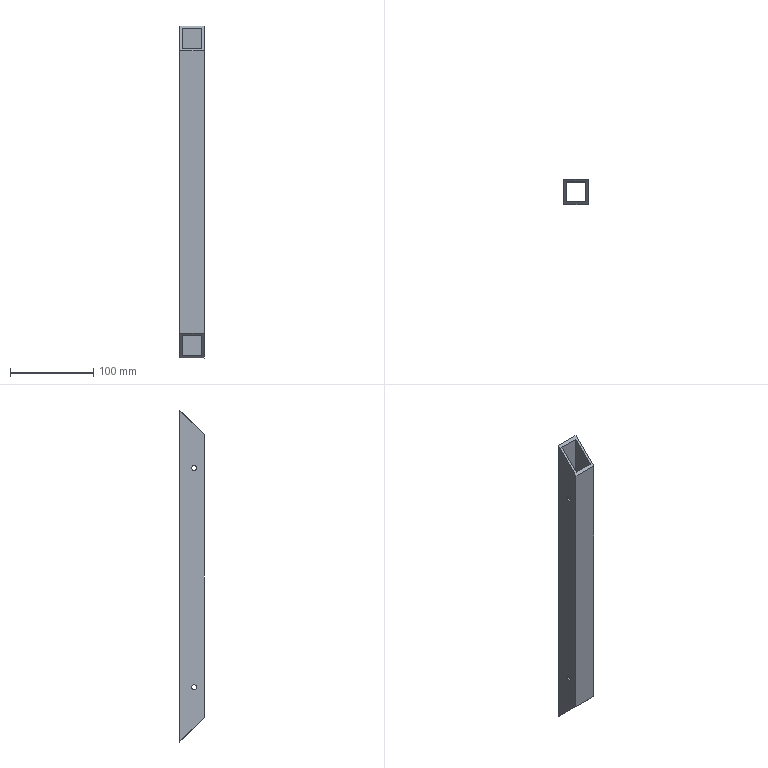Part | SolidWorks | features ICE 4, Extrusion 1 | 1 solid | 18 faces | box 30 x 30 x 400 mm | volume 119541 mm3 | plane 10 | cylinder 8 | commonest cylinder face diameters 6 x8
STEP:
#1=CARTESIAN_POINT('',(-45.142,8.401,333.));
#2=VERTEX_POINT('',#1);
#3=CARTESIAN_POINT('',(-45.142,8.401,327.));
#4=VERTEX_POINT('',#3);
#5=CARTESIAN_POINT('',(-45.142,8.401,330.));
#6=DIRECTION('',(1.,0.,0.));
#7=DIRECTION('',(0.,0.,-1.));
#8=AXIS2_PLACEMENT_3D('',#5,#6,#7);
#9=CIRCLE('',#8,3.);
#10=EDGE_CURVE('',#2,#4,#9,.T.);
#11=ORIENTED_EDGE('',*,*,#10,.F.);
#12=CARTESIAN_POINT('',(-42.142,8.401,333.));
#13=VERTEX_POINT('',#12);
#14=CARTESIAN_POINT('',(-45.142,8.401,333.));
#15=DIRECTION('',(1.,0.,0.));
#16=VECTOR('',#15,1000.);
#17=LINE('',#14,#16);
#18=EDGE_CURVE('',#2,#13,#17,.T.);
#19=ORIENTED_EDGE('',*,*,#18,.T.);
#20=CARTESIAN_POINT('',(-42.142,8.401,327.));
#21=VERTEX_POINT('',#20);
#22=CARTESIAN_POINT('',(-42.142,8.401,330.));
#23=DIRECTION('',(-1.,0.,0.));
#24=DIRECTION('',(0.,0.,1.));
#25=AXIS2_PLACEMENT_3D('',#22,#23,#24);
#26=CIRCLE('',#25,3.);
#27=EDGE_CURVE('',#21,#13,#26,.T.);
#28=ORIENTED_EDGE('',*,*,#27,.F.);
#29=CARTESIAN_POINT('',(-45.142,8.401,327.));
#30=DIRECTION('',(1.,0.,0.));
#31=VECTOR('',#30,1000.);
#32=LINE('',#29,#31);
#33=EDGE_CURVE('',#4,#21,#32,.T.);
#34=ORIENTED_EDGE('',*,*,#33,.F.);
#35=EDGE_LOOP('',(#11,#19,#28,#34));
#36=FACE_OUTER_BOUND('',#35,.T.);
#37=CARTESIAN_POINT('',(-45.142,8.401,330.));
#38=DIRECTION('',(1.,0.,0.));
#39=DIRECTION('',(0.,0.,-1.));
#40=AXIS2_PLACEMENT_3D('',#37,#38,#39);
#41=CYLINDRICAL_SURFACE('',#40,3.);
#42=ADVANCED_FACE('',(#36),#41,.F.);
#43=CARTESIAN_POINT('',(-45.142,8.401,69.));
#44=VERTEX_POINT('',#43);
#45=CARTESIAN_POINT('',(-45.142,8.401,63.));
#46=VERTEX_POINT('',#45);
#47=CARTESIAN_POINT('',(-45.142,8.401,66.));
#48=DIRECTION('',(1.,0.,0.));
#49=DIRECTION('',(0.,0.,-1.));
#50=AXIS2_PLACEMENT_3D('',#47,#48,#49);
#51=CIRCLE('',#50,3.);
#52=EDGE_CURVE('',#44,#46,#51,.T.);
#53=ORIENTED_EDGE('',*,*,#52,.F.);
#54=CARTESIAN_POINT('',(-42.142,8.401,69.));
#55=VERTEX_POINT('',#54);
#56=CARTESIAN_POINT('',(-45.142,8.401,69.));
#57=DIRECTION('',(1.,0.,0.));
#58=VECTOR('',#57,1000.);
#59=LINE('',#56,#58);
#60=EDGE_CURVE('',#44,#55,#59,.T.);
#61=ORIENTED_EDGE('',*,*,#60,.T.);
#62=CARTESIAN_POINT('',(-42.142,8.401,63.));
#63=VERTEX_POINT('',#62);
#64=CARTESIAN_POINT('',(-42.142,8.401,66.));
#65=DIRECTION('',(-1.,0.,0.));
#66=DIRECTION('',(0.,0.,1.));
#67=AXIS2_PLACEMENT_3D('',#64,#65,#66);
#68=CIRCLE('',#67,3.);
#69=EDGE_CURVE('',#63,#55,#68,.T.);
#70=ORIENTED_EDGE('',*,*,#69,.F.);
#71=CARTESIAN_POINT('',(-45.142,8.401,63.));
#72=DIRECTION('',(1.,0.,0.));
#73=VECTOR('',#72,1000.);
#74=LINE('',#71,#73);
#75=EDGE_CURVE('',#46,#63,#74,.T.);
#76=ORIENTED_EDGE('',*,*,#75,.F.);
#77=EDGE_LOOP('',(#53,#61,#70,#76));
#78=FACE_OUTER_BOUND('',#77,.T.);
#79=CARTESIAN_POINT('',(-45.142,8.401,66.));
#80=DIRECTION('',(1.,0.,0.));
#81=DIRECTION('',(0.,0.,-1.));
#82=AXIS2_PLACEMENT_3D('',#79,#80,#81);
#83=CYLINDRICAL_SURFACE('',#82,3.);
#84=ADVANCED_FACE('',(#78),#83,.F.);
#85=CARTESIAN_POINT('',(-18.142,8.401,333.));
#86=VERTEX_POINT('',#85);
#87=CARTESIAN_POINT('',(-18.142,8.401,327.));
#88=VERTEX_POINT('',#87);
#89=CARTESIAN_POINT('',(-18.142,8.401,330.));
#90=DIRECTION('',(1.,0.,0.));
#91=DIRECTION('',(0.,1.,0.));
#92=AXIS2_PLACEMENT_3D('',#89,#90,#91);
#93=CIRCLE('',#92,3.);
#94=EDGE_CURVE('',#86,#88,#93,.T.);
#95=ORIENTED_EDGE('',*,*,#94,.F.);
#96=CARTESIAN_POINT('',(-15.142,8.401,333.));
#97=VERTEX_POINT('',#96);
#98=CARTESIAN_POINT('',(-45.142,8.401,333.));
#99=DIRECTION('',(1.,0.,0.));
#100=VECTOR('',#99,1000.);
#101=LINE('',#98,#100);
#102=EDGE_CURVE('',#86,#97,#101,.T.);
#103=ORIENTED_EDGE('',*,*,#102,.T.);
#104=CARTESIAN_POINT('',(-15.142,8.401,327.));
#105=VERTEX_POINT('',#104);
#106=CARTESIAN_POINT('',(-15.142,8.401,330.));
#107=DIRECTION('',(-1.,0.,0.));
#108=DIRECTION('',(0.,0.,1.));
#109=AXIS2_PLACEMENT_3D('',#106,#107,#108);
#110=CIRCLE('',#109,3.);
#111=EDGE_CURVE('',#105,#97,#110,.T.);
#112=ORIENTED_EDGE('',*,*,#111,.F.);
#113=CARTESIAN_POINT('',(-45.142,8.401,327.));
#114=DIRECTION('',(1.,0.,0.));
#115=VECTOR('',#114,1000.);
#116=LINE('',#113,#115);
#117=EDGE_CURVE('',#88,#105,#116,.T.);
#118=ORIENTED_EDGE('',*,*,#117,.F.);
#119=EDGE_LOOP('',(#95,#103,#112,#118));
#120=FACE_OUTER_BOUND('',#119,.T.);
#121=CARTESIAN_POINT('',(-45.142,8.401,330.));
#122=DIRECTION('',(1.,0.,0.));
#123=DIRECTION('',(0.,0.,-1.));
#124=AXIS2_PLACEMENT_3D('',#121,#122,#123);
#125=CYLINDRICAL_SURFACE('',#124,3.);
#126=ADVANCED_FACE('',(#120),#125,.F.);
#127=CARTESIAN_POINT('',(-18.142,8.401,69.));
#128=VERTEX_POINT('',#127);
#129=CARTESIAN_POINT('',(-18.142,8.401,63.));
#130=VERTEX_POINT('',#129);
#131=CARTESIAN_POINT('',(-18.142,8.401,66.));
#132=DIRECTION('',(1.,0.,0.));
#133=DIRECTION('',(0.,1.,0.));
#134=AXIS2_PLACEMENT_3D('',#131,#132,#133);
#135=CIRCLE('',#134,3.);
#136=EDGE_CURVE('',#128,#130,#135,.T.);
#137=ORIENTED_EDGE('',*,*,#136,.F.);
#138=CARTESIAN_POINT('',(-15.142,8.401,69.));
#139=VERTEX_POINT('',#138);
#140=CARTESIAN_POINT('',(-45.142,8.401,69.));
#141=DIRECTION('',(1.,0.,0.));
#142=VECTOR('',#141,1000.);
#143=LINE('',#140,#142);
#144=EDGE_CURVE('',#128,#139,#143,.T.);
#145=ORIENTED_EDGE('',*,*,#144,.T.);
#146=CARTESIAN_POINT('',(-15.142,8.401,63.));
#147=VERTEX_POINT('',#146);
#148=CARTESIAN_POINT('',(-15.142,8.401,66.));
#149=DIRECTION('',(-1.,0.,0.));
#150=DIRECTION('',(0.,0.,1.));
#151=AXIS2_PLACEMENT_3D('',#148,#149,#150);
#152=CIRCLE('',#151,3.);
#153=EDGE_CURVE('',#147,#139,#152,.T.);
#154=ORIENTED_EDGE('',*,*,#153,.F.);
#155=CARTESIAN_POINT('',(-45.142,8.401,63.));
#156=DIRECTION('',(1.,0.,0.));
#157=VECTOR('',#156,1000.);
#158=LINE('',#155,#157);
#159=EDGE_CURVE('',#130,#147,#158,.T.);
#160=ORIENTED_EDGE('',*,*,#159,.F.);
#161=EDGE_LOOP('',(#137,#145,#154,#160));
#162=FACE_OUTER_BOUND('',#161,.T.);
#163=CARTESIAN_POINT('',(-45.142,8.401,66.));
#164=DIRECTION('',(1.,0.,0.));
#165=DIRECTION('',(0.,0.,-1.));
#166=AXIS2_PLACEMENT_3D('',#163,#164,#165);
#167=CYLINDRICAL_SURFACE('',#166,3.);
#168=ADVANCED_FACE('',(#162),#167,.F.);
#169=CARTESIAN_POINT('',(-45.142,8.401,330.));
#170=DIRECTION('',(1.,0.,0.));
#171=DIRECTION('',(0.,0.,-1.));
#172=AXIS2_PLACEMENT_3D('',#169,#170,#171);
#173=CIRCLE('',#172,3.);
#174=EDGE_CURVE('',#4,#2,#173,.T.);
#175=ORIENTED_EDGE('',*,*,#174,.T.);
#176=ORIENTED_EDGE('',*,*,#10,.T.);
#177=EDGE_LOOP('',(#175,#176));
#178=FACE_BOUND('',#177,.T.);
#179=CARTESIAN_POINT('',(-45.142,8.401,66.));
#180=DIRECTION('',(1.,0.,0.));
#181=DIRECTION('',(0.,0.,-1.));
#182=AXIS2_PLACEMENT_3D('',#179,#180,#181);
#183=CIRCLE('',#182,3.);
#184=EDGE_CURVE('',#46,#44,#183,.T.);
#185=ORIENTED_EDGE('',*,*,#184,.T.);
#186=ORIENTED_EDGE('',*,*,#52,.T.);
#187=EDGE_LOOP('',(#185,#186));
#188=FACE_BOUND('',#187,.T.);
#189=CARTESIAN_POINT('',(-45.142,-4.099,370.));
#190=VERTEX_POINT('',#189);
#191=CARTESIAN_POINT('',(-45.142,-4.099,30.));
#192=VERTEX_POINT('',#191);
#193=CARTESIAN_POINT('',(-45.142,-4.099,400.));
#194=DIRECTION('',(0.,0.,-1.));
#195=VECTOR('',#194,1000.);
#196=LINE('',#193,#195);
#197=EDGE_CURVE('',#190,#192,#196,.T.);
#198=ORIENTED_EDGE('',*,*,#197,.F.);
#199=CARTESIAN_POINT('',(-45.142,25.901,400.));
#200=VERTEX_POINT('',#199);
#201=CARTESIAN_POINT('',(-45.142,25.901,400.));
#202=DIRECTION('',(0.,0.7071,0.7071));
#203=VECTOR('',#202,1000.);
#204=LINE('',#201,#203);
#205=EDGE_CURVE('',#190,#200,#204,.T.);
#206=ORIENTED_EDGE('',*,*,#205,.T.);
#207=CARTESIAN_POINT('',(-45.142,25.901,0.));
#208=VERTEX_POINT('',#207);
#209=CARTESIAN_POINT('',(-45.142,25.901,400.));
#210=DIRECTION('',(0.,0.,-1.));
#211=VECTOR('',#210,1000.);
#212=LINE('',#209,#211);
#213=EDGE_CURVE('',#200,#208,#212,.T.);
#214=ORIENTED_EDGE('',*,*,#213,.T.);
#215=CARTESIAN_POINT('',(-45.142,25.901,0.));
#216=DIRECTION('',(0.,-0.7071,0.7071));
#217=VECTOR('',#216,1000.);
#218=LINE('',#215,#217);
#219=EDGE_CURVE('',#208,#192,#218,.T.);
#220=ORIENTED_EDGE('',*,*,#219,.T.);
#221=EDGE_LOOP('',(#198,#206,#214,#220));
#222=FACE_OUTER_BOUND('',#221,.T.);
#223=CARTESIAN_POINT('',(-45.142,-4.099,400.));
#224=DIRECTION('',(1.,0.,0.));
#225=DIRECTION('',(0.,0.,-1.));
#226=AXIS2_PLACEMENT_3D('',#223,#224,#225);
#227=PLANE('',#226);
#228=ADVANCED_FACE('',(#178,#188,#222),#227,.F.);
#229=CARTESIAN_POINT('',(-15.142,-4.099,370.));
#230=VERTEX_POINT('',#229);
#231=CARTESIAN_POINT('',(-15.142,-4.099,30.));
#232=VERTEX_POINT('',#231);
#233=CARTESIAN_POINT('',(-15.142,-4.099,400.));
#234=DIRECTION('',(0.,0.,-1.));
#235=VECTOR('',#234,1000.);
#236=LINE('',#233,#235);
#237=EDGE_CURVE('',#230,#232,#236,.T.);
#238=ORIENTED_EDGE('',*,*,#237,.F.);
#239=CARTESIAN_POINT('',(-45.142,-4.099,370.));
#240=DIRECTION('',(1.,0.,0.));
#241=VECTOR('',#240,1000.);
#242=LINE('',#239,#241);
#243=EDGE_CURVE('',#190,#230,#242,.T.);
#244=ORIENTED_EDGE('',*,*,#243,.F.);
#245=ORIENTED_EDGE('',*,*,#197,.T.);
#246=CARTESIAN_POINT('',(-45.142,-4.099,30.));
#247=DIRECTION('',(1.,0.,0.));
#248=VECTOR('',#247,1000.);
#249=LINE('',#246,#248);
#250=EDGE_CURVE('',#192,#232,#249,.T.);
#251=ORIENTED_EDGE('',*,*,#250,.T.);
#252=EDGE_LOOP('',(#238,#244,#245,#251));
#253=FACE_OUTER_BOUND('',#252,.T.);
#254=CARTESIAN_POINT('',(-15.142,-4.099,400.));
#255=DIRECTION('',(0.,1.,0.));
#256=DIRECTION('',(0.,0.,1.));
#257=AXIS2_PLACEMENT_3D('',#254,#255,#256);
#258=PLANE('',#257);
#259=ADVANCED_FACE('',(#253),#258,.F.);
#260=ORIENTED_EDGE('',*,*,#111,.T.);
#261=CARTESIAN_POINT('',(-15.142,8.401,330.));
#262=DIRECTION('',(-1.,0.,0.));
#263=DIRECTION('',(0.,0.,1.));
#264=AXIS2_PLACEMENT_3D('',#261,#262,#263);
#265=CIRCLE('',#264,3.);
#266=EDGE_CURVE('',#97,#105,#265,.T.);
#267=ORIENTED_EDGE('',*,*,#266,.T.);
#268=EDGE_LOOP('',(#260,#267));
#269=FACE_BOUND('',#268,.T.);
#270=ORIENTED_EDGE('',*,*,#153,.T.);
#271=CARTESIAN_POINT('',(-15.142,8.401,66.));
#272=DIRECTION('',(-1.,0.,0.));
#273=DIRECTION('',(0.,0.,1.));
#274=AXIS2_PLACEMENT_3D('',#271,#272,#273);
#275=CIRCLE('',#274,3.);
#276=EDGE_CURVE('',#139,#147,#275,.T.);
#277=ORIENTED_EDGE('',*,*,#276,.T.);
#278=EDGE_LOOP('',(#270,#277));
#279=FACE_BOUND('',#278,.T.);
#280=CARTESIAN_POINT('',(-15.142,25.901,400.));
#281=VERTEX_POINT('',#280);
#282=CARTESIAN_POINT('',(-15.142,25.901,0.));
#283=VERTEX_POINT('',#282);
#284=CARTESIAN_POINT('',(-15.142,25.901,400.));
#285=DIRECTION('',(0.,0.,-1.));
#286=VECTOR('',#285,1000.);
#287=LINE('',#284,#286);
#288=EDGE_CURVE('',#281,#283,#287,.T.);
#289=ORIENTED_EDGE('',*,*,#288,.F.);
#290=CARTESIAN_POINT('',(-15.142,25.901,400.));
#291=DIRECTION('',(0.,0.7071,0.7071));
#292=VECTOR('',#291,1000.);
#293=LINE('',#290,#292);
#294=EDGE_CURVE('',#230,#281,#293,.T.);
#295=ORIENTED_EDGE('',*,*,#294,.F.);
#296=ORIENTED_EDGE('',*,*,#237,.T.);
#297=CARTESIAN_POINT('',(-15.142,25.901,0.));
#298=DIRECTION('',(0.,-0.7071,0.7071));
#299=VECTOR('',#298,1000.);
#300=LINE('',#297,#299);
#301=EDGE_CURVE('',#283,#232,#300,.T.);
#302=ORIENTED_EDGE('',*,*,#301,.F.);
#303=EDGE_LOOP('',(#289,#295,#296,#302));
#304=FACE_OUTER_BOUND('',#303,.T.);
#305=CARTESIAN_POINT('',(-15.142,25.901,400.));
#306=DIRECTION('',(-1.,0.,0.));
#307=DIRECTION('',(0.,0.,1.));
#308=AXIS2_PLACEMENT_3D('',#305,#306,#307);
#309=PLANE('',#308);
#310=ADVANCED_FACE('',(#269,#279,#304),#309,.F.);
#311=CARTESIAN_POINT('',(-45.142,25.901,0.));
#312=DIRECTION('',(-1.,0.,0.));
#313=VECTOR('',#312,1000.);
#314=LINE('',#311,#313);
#315=EDGE_CURVE('',#283,#208,#314,.T.);
#316=ORIENTED_EDGE('',*,*,#315,.T.);
#317=ORIENTED_EDGE('',*,*,#213,.F.);
#318=CARTESIAN_POINT('',(-45.142,25.901,400.));
#319=DIRECTION('',(-1.,0.,0.));
#320=VECTOR('',#319,1000.);
#321=LINE('',#318,#320);
#322=EDGE_CURVE('',#281,#200,#321,.T.);
#323=ORIENTED_EDGE('',*,*,#322,.F.);
#324=ORIENTED_EDGE('',*,*,#288,.T.);
#325=EDGE_LOOP('',(#316,#317,#323,#324));
#326=FACE_OUTER_BOUND('',#325,.T.);
#327=CARTESIAN_POINT('',(-45.142,25.901,400.));
#328=DIRECTION('',(0.,-1.,0.));
#329=DIRECTION('',(0.,0.,-1.));
#330=AXIS2_PLACEMENT_3D('',#327,#328,#329);
#331=PLANE('',#330);
#332=ADVANCED_FACE('',(#326),#331,.F.);
#333=ORIENTED_EDGE('',*,*,#27,.T.);
#334=CARTESIAN_POINT('',(-42.142,8.401,330.));
#335=DIRECTION('',(-1.,0.,0.));
#336=DIRECTION('',(0.,0.,1.));
#337=AXIS2_PLACEMENT_3D('',#334,#335,#336);
#338=CIRCLE('',#337,3.);
#339=EDGE_CURVE('',#13,#21,#338,.T.);
#340=ORIENTED_EDGE('',*,*,#339,.T.);
#341=EDGE_LOOP('',(#333,#340));
#342=FACE_BOUND('',#341,.T.);
#343=ORIENTED_EDGE('',*,*,#69,.T.);
#344=CARTESIAN_POINT('',(-42.142,8.401,66.));
#345=DIRECTION('',(-1.,0.,0.));
#346=DIRECTION('',(0.,0.,1.));
#347=AXIS2_PLACEMENT_3D('',#344,#345,#346);
#348=CIRCLE('',#347,3.);
#349=EDGE_CURVE('',#55,#63,#348,.T.);
#350=ORIENTED_EDGE('',*,*,#349,.T.);
#351=EDGE_LOOP('',(#343,#350));
#352=FACE_BOUND('',#351,.T.);
#353=CARTESIAN_POINT('',(-42.142,22.901,3.));
#354=VERTEX_POINT('',#353);
#355=CARTESIAN_POINT('',(-42.142,22.901,397.));
#356=VERTEX_POINT('',#355);
#357=CARTESIAN_POINT('',(-42.142,22.901,-92.));
#358=DIRECTION('',(0.,0.,1.));
#359=VECTOR('',#358,1000.);
#360=LINE('',#357,#359);
#361=EDGE_CURVE('',#354,#356,#360,.T.);
#362=ORIENTED_EDGE('',*,*,#361,.T.);
#363=CARTESIAN_POINT('',(-42.142,-1.099,373.));
#364=VERTEX_POINT('',#363);
#365=CARTESIAN_POINT('',(-42.142,-233.599,140.5));
#366=DIRECTION('',(0.,-0.7071,-0.7071));
#367=VECTOR('',#366,1000.);
#368=LINE('',#365,#367);
#369=EDGE_CURVE('',#356,#364,#368,.T.);
#370=ORIENTED_EDGE('',*,*,#369,.T.);
#371=CARTESIAN_POINT('',(-42.142,-1.099,27.));
#372=VERTEX_POINT('',#371);
#373=CARTESIAN_POINT('',(-42.142,-1.099,-92.));
#374=DIRECTION('',(0.,0.,1.));
#375=VECTOR('',#374,1000.);
#376=LINE('',#373,#375);
#377=EDGE_CURVE('',#372,#364,#376,.T.);
#378=ORIENTED_EDGE('',*,*,#377,.F.);
#379=CARTESIAN_POINT('',(-42.142,58.401,-32.5));
#380=DIRECTION('',(0.,0.7071,-0.7071));
#381=VECTOR('',#380,1000.);
#382=LINE('',#379,#381);
#383=EDGE_CURVE('',#372,#354,#382,.T.);
#384=ORIENTED_EDGE('',*,*,#383,.T.);
#385=EDGE_LOOP('',(#362,#370,#378,#384));
#386=FACE_OUTER_BOUND('',#385,.T.);
#387=CARTESIAN_POINT('',(-42.142,-1.099,-92.));
#388=DIRECTION('',(-1.,0.,0.));
#389=DIRECTION('',(0.,0.,1.));
#390=AXIS2_PLACEMENT_3D('',#387,#388,#389);
#391=PLANE('',#390);
#392=ADVANCED_FACE('',(#342,#352,#386),#391,.F.);
#393=CARTESIAN_POINT('',(-18.142,22.901,3.));
#394=VERTEX_POINT('',#393);
#395=CARTESIAN_POINT('',(-18.142,22.901,397.));
#396=VERTEX_POINT('',#395);
#397=CARTESIAN_POINT('',(-18.142,22.901,-92.));
#398=DIRECTION('',(0.,0.,1.));
#399=VECTOR('',#398,1000.);
#400=LINE('',#397,#399);
#401=EDGE_CURVE('',#394,#396,#400,.T.);
#402=ORIENTED_EDGE('',*,*,#401,.T.);
#403=CARTESIAN_POINT('',(-42.142,22.901,397.));
#404=DIRECTION('',(-1.,0.,0.));
#405=VECTOR('',#404,1000.);
#406=LINE('',#403,#405);
#407=EDGE_CURVE('',#396,#356,#406,.T.);
#408=ORIENTED_EDGE('',*,*,#407,.T.);
#409=ORIENTED_EDGE('',*,*,#361,.F.);
#410=CARTESIAN_POINT('',(-42.142,22.901,3.));
#411=DIRECTION('',(1.,0.,0.));
#412=VECTOR('',#411,1000.);
#413=LINE('',#410,#412);
#414=EDGE_CURVE('',#354,#394,#413,.T.);
#415=ORIENTED_EDGE('',*,*,#414,.T.);
#416=EDGE_LOOP('',(#402,#408,#409,#415));
#417=FACE_OUTER_BOUND('',#416,.T.);
#418=CARTESIAN_POINT('',(-42.142,22.901,-92.));
#419=DIRECTION('',(0.,1.,0.));
#420=DIRECTION('',(0.,0.,1.));
#421=AXIS2_PLACEMENT_3D('',#418,#419,#420);
#422=PLANE('',#421);
#423=ADVANCED_FACE('',(#417),#422,.F.);
#424=CARTESIAN_POINT('',(-18.142,8.401,330.));
#425=DIRECTION('',(1.,0.,0.));
#426=DIRECTION('',(0.,1.,0.));
#427=AXIS2_PLACEMENT_3D('',#424,#425,#426);
#428=CIRCLE('',#427,3.);
#429=EDGE_CURVE('',#88,#86,#428,.T.);
#430=ORIENTED_EDGE('',*,*,#429,.T.);
#431=ORIENTED_EDGE('',*,*,#94,.T.);
#432=EDGE_LOOP('',(#430,#431));
#433=FACE_BOUND('',#432,.T.);
#434=CARTESIAN_POINT('',(-18.142,8.401,66.));
#435=DIRECTION('',(1.,0.,0.));
#436=DIRECTION('',(0.,1.,0.));
#437=AXIS2_PLACEMENT_3D('',#434,#435,#436);
#438=CIRCLE('',#437,3.);
#439=EDGE_CURVE('',#130,#128,#438,.T.);
#440=ORIENTED_EDGE('',*,*,#439,.T.);
#441=ORIENTED_EDGE('',*,*,#136,.T.);
#442=EDGE_LOOP('',(#440,#441));
#443=FACE_BOUND('',#442,.T.);
#444=CARTESIAN_POINT('',(-18.142,-1.099,27.));
#445=VERTEX_POINT('',#444);
#446=CARTESIAN_POINT('',(-18.142,-1.099,373.));
#447=VERTEX_POINT('',#446);
#448=CARTESIAN_POINT('',(-18.142,-1.099,-92.));
#449=DIRECTION('',(0.,0.,1.));
#450=VECTOR('',#449,1000.);
#451=LINE('',#448,#450);
#452=EDGE_CURVE('',#445,#447,#451,.T.);
#453=ORIENTED_EDGE('',*,*,#452,.T.);
#454=CARTESIAN_POINT('',(-18.142,-221.599,152.5));
#455=DIRECTION('',(0.,0.7071,0.7071));
#456=VECTOR('',#455,1000.);
#457=LINE('',#454,#456);
#458=EDGE_CURVE('',#447,#396,#457,.T.);
#459=ORIENTED_EDGE('',*,*,#458,.T.);
#460=ORIENTED_EDGE('',*,*,#401,.F.);
#461=CARTESIAN_POINT('',(-18.142,70.401,-44.5));
#462=DIRECTION('',(0.,-0.7071,0.7071));
#463=VECTOR('',#462,1000.);
#464=LINE('',#461,#463);
#465=EDGE_CURVE('',#394,#445,#464,.T.);
#466=ORIENTED_EDGE('',*,*,#465,.T.);
#467=EDGE_LOOP('',(#453,#459,#460,#466));
#468=FACE_OUTER_BOUND('',#467,.T.);
#469=CARTESIAN_POINT('',(-18.142,22.901,-92.));
#470=DIRECTION('',(1.,0.,0.));
#471=DIRECTION('',(0.,1.,0.));
#472=AXIS2_PLACEMENT_3D('',#469,#470,#471);
#473=PLANE('',#472);
#474=ADVANCED_FACE('',(#433,#443,#468),#473,.F.);
#475=ORIENTED_EDGE('',*,*,#377,.T.);
#476=CARTESIAN_POINT('',(-18.142,-1.099,373.));
#477=DIRECTION('',(1.,0.,0.));
#478=VECTOR('',#477,1000.);
#479=LINE('',#476,#478);
#480=EDGE_CURVE('',#364,#447,#479,.T.);
#481=ORIENTED_EDGE('',*,*,#480,.T.);
#482=ORIENTED_EDGE('',*,*,#452,.F.);
#483=CARTESIAN_POINT('',(-18.142,-1.099,27.));
#484=DIRECTION('',(-1.,0.,0.));
#485=VECTOR('',#484,1000.);
#486=LINE('',#483,#485);
#487=EDGE_CURVE('',#445,#372,#486,.T.);
#488=ORIENTED_EDGE('',*,*,#487,.T.);
#489=EDGE_LOOP('',(#475,#481,#482,#488));
#490=FACE_OUTER_BOUND('',#489,.T.);
#491=CARTESIAN_POINT('',(-18.142,-1.099,-92.));
#492=DIRECTION('',(0.,-1.,0.));
#493=DIRECTION('',(1.,0.,0.));
#494=AXIS2_PLACEMENT_3D('',#491,#492,#493);
#495=PLANE('',#494);
#496=ADVANCED_FACE('',(#490),#495,.F.);
#497=ORIENTED_EDGE('',*,*,#301,.T.);
#498=ORIENTED_EDGE('',*,*,#250,.F.);
#499=ORIENTED_EDGE('',*,*,#219,.F.);
#500=ORIENTED_EDGE('',*,*,#315,.F.);
#501=EDGE_LOOP('',(#497,#498,#499,#500));
#502=FACE_OUTER_BOUND('',#501,.T.);
#503=ORIENTED_EDGE('',*,*,#487,.F.);
#504=ORIENTED_EDGE('',*,*,#465,.F.);
#505=ORIENTED_EDGE('',*,*,#414,.F.);
#506=ORIENTED_EDGE('',*,*,#383,.F.);
#507=EDGE_LOOP('',(#503,#504,#505,#506));
#508=FACE_BOUND('',#507,.T.);
#509=CARTESIAN_POINT('',(-45.142,25.901,0.));
#510=DIRECTION('',(0.,0.7071,0.7071));
#511=DIRECTION('',(0.,-0.7071,0.7071));
#512=AXIS2_PLACEMENT_3D('',#509,#510,#511);
#513=PLANE('',#512);
#514=ADVANCED_FACE('',(#502,#508),#513,.F.);
#515=ORIENTED_EDGE('',*,*,#294,.T.);
#516=ORIENTED_EDGE('',*,*,#322,.T.);
#517=ORIENTED_EDGE('',*,*,#205,.F.);
#518=ORIENTED_EDGE('',*,*,#243,.T.);
#519=EDGE_LOOP('',(#515,#516,#517,#518));
#520=FACE_OUTER_BOUND('',#519,.T.);
#521=ORIENTED_EDGE('',*,*,#407,.F.);
#522=ORIENTED_EDGE('',*,*,#458,.F.);
#523=ORIENTED_EDGE('',*,*,#480,.F.);
#524=ORIENTED_EDGE('',*,*,#369,.F.);
#525=EDGE_LOOP('',(#521,#522,#523,#524));
#526=FACE_BOUND('',#525,.T.);
#527=CARTESIAN_POINT('',(-45.142,25.901,400.));
#528=DIRECTION('',(0.,0.7071,-0.7071));
#529=DIRECTION('',(0.,0.7071,0.7071));
#530=AXIS2_PLACEMENT_3D('',#527,#528,#529);
#531=PLANE('',#530);
#532=ADVANCED_FACE('',(#520,#526),#531,.F.);
#533=ORIENTED_EDGE('',*,*,#144,.F.);
#534=ORIENTED_EDGE('',*,*,#439,.F.);
#535=ORIENTED_EDGE('',*,*,#159,.T.);
#536=ORIENTED_EDGE('',*,*,#276,.F.);
#537=EDGE_LOOP('',(#533,#534,#535,#536));
#538=FACE_OUTER_BOUND('',#537,.T.);
#539=CARTESIAN_POINT('',(-45.142,8.401,66.));
#540=DIRECTION('',(1.,0.,0.));
#541=DIRECTION('',(0.,0.,-1.));
#542=AXIS2_PLACEMENT_3D('',#539,#540,#541);
#543=CYLINDRICAL_SURFACE('',#542,3.);
#544=ADVANCED_FACE('',(#538),#543,.F.);
#545=ORIENTED_EDGE('',*,*,#102,.F.);
#546=ORIENTED_EDGE('',*,*,#429,.F.);
#547=ORIENTED_EDGE('',*,*,#117,.T.);
#548=ORIENTED_EDGE('',*,*,#266,.F.);
#549=EDGE_LOOP('',(#545,#546,#547,#548));
#550=FACE_OUTER_BOUND('',#549,.T.);
#551=CARTESIAN_POINT('',(-45.142,8.401,330.));
#552=DIRECTION('',(1.,0.,0.));
#553=DIRECTION('',(0.,0.,-1.));
#554=AXIS2_PLACEMENT_3D('',#551,#552,#553);
#555=CYLINDRICAL_SURFACE('',#554,3.);
#556=ADVANCED_FACE('',(#550),#555,.F.);
#557=ORIENTED_EDGE('',*,*,#60,.F.);
#558=ORIENTED_EDGE('',*,*,#184,.F.);
#559=ORIENTED_EDGE('',*,*,#75,.T.);
#560=ORIENTED_EDGE('',*,*,#349,.F.);
#561=EDGE_LOOP('',(#557,#558,#559,#560));
#562=FACE_OUTER_BOUND('',#561,.T.);
#563=CARTESIAN_POINT('',(-45.142,8.401,66.));
#564=DIRECTION('',(1.,0.,0.));
#565=DIRECTION('',(0.,0.,-1.));
#566=AXIS2_PLACEMENT_3D('',#563,#564,#565);
#567=CYLINDRICAL_SURFACE('',#566,3.);
#568=ADVANCED_FACE('',(#562),#567,.F.);
#569=ORIENTED_EDGE('',*,*,#18,.F.);
#570=ORIENTED_EDGE('',*,*,#174,.F.);
#571=ORIENTED_EDGE('',*,*,#33,.T.);
#572=ORIENTED_EDGE('',*,*,#339,.F.);
#573=EDGE_LOOP('',(#569,#570,#571,#572));
#574=FACE_OUTER_BOUND('',#573,.T.);
#575=CARTESIAN_POINT('',(-45.142,8.401,330.));
#576=DIRECTION('',(1.,0.,0.));
#577=DIRECTION('',(0.,0.,-1.));
#578=AXIS2_PLACEMENT_3D('',#575,#576,#577);
#579=CYLINDRICAL_SURFACE('',#578,3.);
#580=ADVANCED_FACE('',(#574),#579,.F.);
#581=CLOSED_SHELL('',(#42,#84,#126,#168,#228,#259,#310,#332,#392,#423,#474,#496,#514,#532,#544,#556,#568,#580));
#582=MANIFOLD_SOLID_BREP('',#581);
#583=CARTESIAN_POINT('',(0.,0.,0.));
#584=DIRECTION('',(0.,0.,1.));
#585=DIRECTION('',(1.,0.,0.));
#586=AXIS2_PLACEMENT_3D('',#583,#584,#585);
#587=(LENGTH_UNIT()NAMED_UNIT(*)SI_UNIT(.MILLI.,.METRE.));
#588=UNCERTAINTY_MEASURE_WITH_UNIT(LENGTH_MEASURE(0.00001),#587,'','');
#589=(NAMED_UNIT(*)PLANE_ANGLE_UNIT()SI_UNIT($,.RADIAN.));
#590=(NAMED_UNIT(*)SI_UNIT($,.STERADIAN.)SOLID_ANGLE_UNIT());
#591=(GEOMETRIC_REPRESENTATION_CONTEXT(3)GLOBAL_UNCERTAINTY_ASSIGNED_CONTEXT((#588))GLOBAL_UNIT_ASSIGNED_CONTEXT((#587,#589,#590))REPRESENTATION_CONTEXT('',''));
#592=ADVANCED_BREP_SHAPE_REPRESENTATION('',(#582,#586),#591);